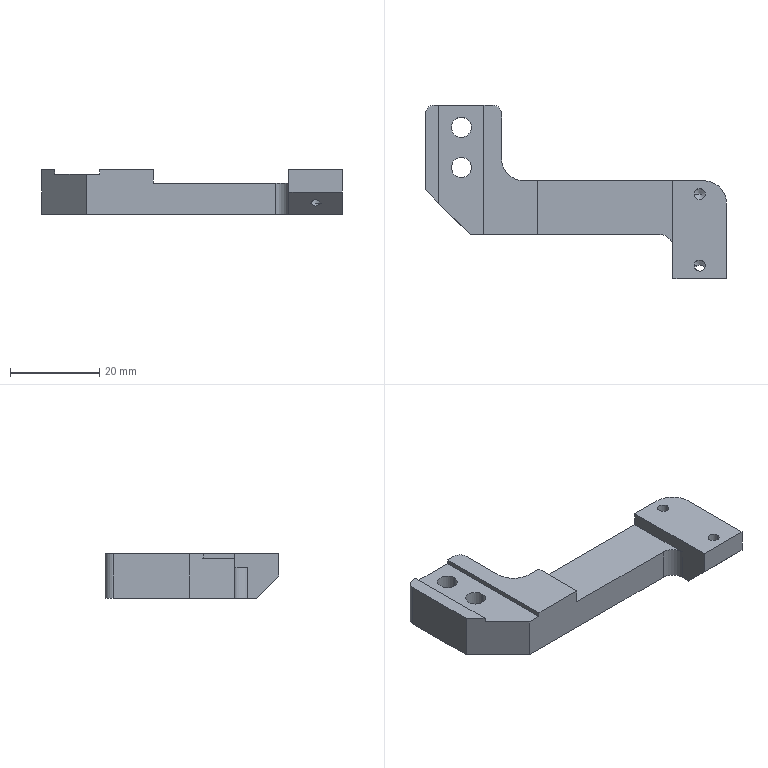Part | STEP file | PN_0059 | 1 solid | 37 faces | box 67.5 x 39 x 10 mm | volume 9820 mm3 | plane 19 | cylinder 13 | cone 5 | commonest cylinder face diameters 2.5 x4 4.5 x4 4 x2 10 x2 6 x1